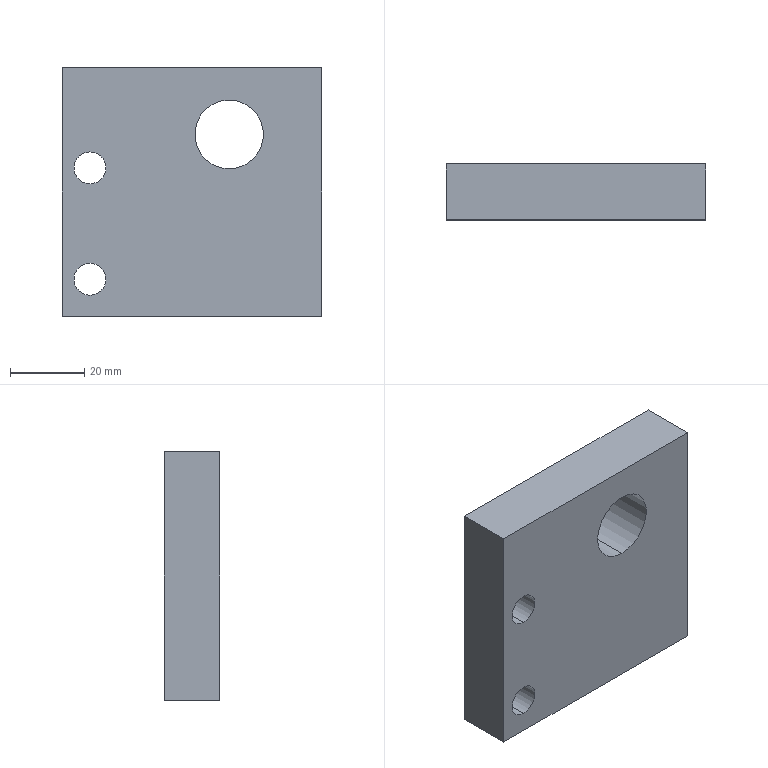Part | 1 solid | 12 faces | box 70 x 15 x 67 mm | volume 64575 mm3 | cylinder 6 | plane 6 | commonest cylinder face diameters 8.6 x4 18.5 x2
STEP:
#1=CARTESIAN_POINT('',(10.,0.,6.25));
#2=VERTEX_POINT('',#1);
#3=CARTESIAN_POINT('',(10.,0.,24.75));
#4=VERTEX_POINT('',#3);
#5=CARTESIAN_POINT('',(10.,0.,15.5));
#6=DIRECTION('',(0.,1.,0.));
#7=DIRECTION('',(0.,0.,1.));
#8=AXIS2_PLACEMENT_3D('',#5,#6,#7);
#9=CIRCLE('',#8,9.25);
#10=EDGE_CURVE('',#2,#4,#9,.T.);
#11=ORIENTED_EDGE('',*,*,#10,.F.);
#12=CARTESIAN_POINT('',(10.,15.,6.25));
#13=VERTEX_POINT('',#12);
#14=CARTESIAN_POINT('',(10.,15.,6.25));
#15=DIRECTION('',(0.,1.,0.));
#16=VECTOR('',#15,1000.);
#17=LINE('',#14,#16);
#18=EDGE_CURVE('',#2,#13,#17,.T.);
#19=ORIENTED_EDGE('',*,*,#18,.T.);
#20=CARTESIAN_POINT('',(10.,15.,24.75));
#21=VERTEX_POINT('',#20);
#22=CARTESIAN_POINT('',(10.,15.,15.5));
#23=DIRECTION('',(0.,1.,0.));
#24=DIRECTION('',(0.,0.,1.));
#25=AXIS2_PLACEMENT_3D('',#22,#23,#24);
#26=CIRCLE('',#25,9.25);
#27=EDGE_CURVE('',#13,#21,#26,.T.);
#28=ORIENTED_EDGE('',*,*,#27,.T.);
#29=CARTESIAN_POINT('',(10.,15.,24.75));
#30=DIRECTION('',(0.,1.,0.));
#31=VECTOR('',#30,1000.);
#32=LINE('',#29,#31);
#33=EDGE_CURVE('',#4,#21,#32,.T.);
#34=ORIENTED_EDGE('',*,*,#33,.F.);
#35=EDGE_LOOP('',(#11,#19,#28,#34));
#36=FACE_OUTER_BOUND('',#35,.T.);
#37=CARTESIAN_POINT('',(10.,15.,15.5));
#38=DIRECTION('',(0.,1.,0.));
#39=DIRECTION('',(0.,0.,1.));
#40=AXIS2_PLACEMENT_3D('',#37,#38,#39);
#41=CYLINDRICAL_SURFACE('',#40,9.25);
#42=ADVANCED_FACE('',(#36),#41,.F.);
#43=CARTESIAN_POINT('',(-27.5,0.,-27.8));
#44=VERTEX_POINT('',#43);
#45=CARTESIAN_POINT('',(-27.5,0.,-19.2));
#46=VERTEX_POINT('',#45);
#47=CARTESIAN_POINT('',(-27.5,0.,-23.5));
#48=DIRECTION('',(0.,1.,0.));
#49=DIRECTION('',(0.,0.,1.));
#50=AXIS2_PLACEMENT_3D('',#47,#48,#49);
#51=CIRCLE('',#50,4.3);
#52=EDGE_CURVE('',#44,#46,#51,.T.);
#53=ORIENTED_EDGE('',*,*,#52,.F.);
#54=CARTESIAN_POINT('',(-27.5,15.,-27.8));
#55=VERTEX_POINT('',#54);
#56=CARTESIAN_POINT('',(-27.5,0.,-27.8));
#57=DIRECTION('',(0.,1.,0.));
#58=VECTOR('',#57,1000.);
#59=LINE('',#56,#58);
#60=EDGE_CURVE('',#44,#55,#59,.T.);
#61=ORIENTED_EDGE('',*,*,#60,.T.);
#62=CARTESIAN_POINT('',(-27.5,15.,-19.2));
#63=VERTEX_POINT('',#62);
#64=CARTESIAN_POINT('',(-27.5,15.,-23.5));
#65=DIRECTION('',(0.,1.,0.));
#66=DIRECTION('',(0.,0.,1.));
#67=AXIS2_PLACEMENT_3D('',#64,#65,#66);
#68=CIRCLE('',#67,4.3);
#69=EDGE_CURVE('',#55,#63,#68,.T.);
#70=ORIENTED_EDGE('',*,*,#69,.T.);
#71=CARTESIAN_POINT('',(-27.5,0.,-19.2));
#72=DIRECTION('',(0.,1.,0.));
#73=VECTOR('',#72,1000.);
#74=LINE('',#71,#73);
#75=EDGE_CURVE('',#46,#63,#74,.T.);
#76=ORIENTED_EDGE('',*,*,#75,.F.);
#77=EDGE_LOOP('',(#53,#61,#70,#76));
#78=FACE_OUTER_BOUND('',#77,.T.);
#79=CARTESIAN_POINT('',(-27.5,0.,-23.5));
#80=DIRECTION('',(0.,1.,0.));
#81=DIRECTION('',(0.,0.,1.));
#82=AXIS2_PLACEMENT_3D('',#79,#80,#81);
#83=CYLINDRICAL_SURFACE('',#82,4.3);
#84=ADVANCED_FACE('',(#78),#83,.F.);
#85=CARTESIAN_POINT('',(-27.5,0.,2.2));
#86=VERTEX_POINT('',#85);
#87=CARTESIAN_POINT('',(-27.5,0.,10.8));
#88=VERTEX_POINT('',#87);
#89=CARTESIAN_POINT('',(-27.5,0.,6.5));
#90=DIRECTION('',(0.,1.,0.));
#91=DIRECTION('',(0.,0.,1.));
#92=AXIS2_PLACEMENT_3D('',#89,#90,#91);
#93=CIRCLE('',#92,4.3);
#94=EDGE_CURVE('',#86,#88,#93,.T.);
#95=ORIENTED_EDGE('',*,*,#94,.F.);
#96=CARTESIAN_POINT('',(-27.5,15.,2.2));
#97=VERTEX_POINT('',#96);
#98=CARTESIAN_POINT('',(-27.5,0.,2.2));
#99=DIRECTION('',(0.,1.,0.));
#100=VECTOR('',#99,1000.);
#101=LINE('',#98,#100);
#102=EDGE_CURVE('',#86,#97,#101,.T.);
#103=ORIENTED_EDGE('',*,*,#102,.T.);
#104=CARTESIAN_POINT('',(-27.5,15.,10.8));
#105=VERTEX_POINT('',#104);
#106=CARTESIAN_POINT('',(-27.5,15.,6.5));
#107=DIRECTION('',(0.,1.,0.));
#108=DIRECTION('',(0.,0.,1.));
#109=AXIS2_PLACEMENT_3D('',#106,#107,#108);
#110=CIRCLE('',#109,4.3);
#111=EDGE_CURVE('',#97,#105,#110,.T.);
#112=ORIENTED_EDGE('',*,*,#111,.T.);
#113=CARTESIAN_POINT('',(-27.5,0.,10.8));
#114=DIRECTION('',(0.,1.,0.));
#115=VECTOR('',#114,1000.);
#116=LINE('',#113,#115);
#117=EDGE_CURVE('',#88,#105,#116,.T.);
#118=ORIENTED_EDGE('',*,*,#117,.F.);
#119=EDGE_LOOP('',(#95,#103,#112,#118));
#120=FACE_OUTER_BOUND('',#119,.T.);
#121=CARTESIAN_POINT('',(-27.5,0.,6.5));
#122=DIRECTION('',(0.,1.,0.));
#123=DIRECTION('',(0.,0.,1.));
#124=AXIS2_PLACEMENT_3D('',#121,#122,#123);
#125=CYLINDRICAL_SURFACE('',#124,4.3);
#126=ADVANCED_FACE('',(#120),#125,.F.);
#127=CARTESIAN_POINT('',(35.,0.,33.5));
#128=VERTEX_POINT('',#127);
#129=CARTESIAN_POINT('',(35.,0.,-33.5));
#130=VERTEX_POINT('',#129);
#131=CARTESIAN_POINT('',(35.,0.,33.5));
#132=DIRECTION('',(0.,0.,-1.));
#133=VECTOR('',#132,1000.);
#134=LINE('',#131,#133);
#135=EDGE_CURVE('',#128,#130,#134,.T.);
#136=ORIENTED_EDGE('',*,*,#135,.T.);
#137=CARTESIAN_POINT('',(35.,15.,-33.5));
#138=VERTEX_POINT('',#137);
#139=CARTESIAN_POINT('',(35.,15.,-33.5));
#140=DIRECTION('',(0.,-1.,0.));
#141=VECTOR('',#140,1000.);
#142=LINE('',#139,#141);
#143=EDGE_CURVE('',#138,#130,#142,.T.);
#144=ORIENTED_EDGE('',*,*,#143,.F.);
#145=CARTESIAN_POINT('',(35.,15.,33.5));
#146=VERTEX_POINT('',#145);
#147=CARTESIAN_POINT('',(35.,15.,33.5));
#148=DIRECTION('',(0.,0.,-1.));
#149=VECTOR('',#148,1000.);
#150=LINE('',#147,#149);
#151=EDGE_CURVE('',#146,#138,#150,.T.);
#152=ORIENTED_EDGE('',*,*,#151,.F.);
#153=CARTESIAN_POINT('',(35.,15.,33.5));
#154=DIRECTION('',(0.,-1.,0.));
#155=VECTOR('',#154,1000.);
#156=LINE('',#153,#155);
#157=EDGE_CURVE('',#146,#128,#156,.T.);
#158=ORIENTED_EDGE('',*,*,#157,.T.);
#159=EDGE_LOOP('',(#136,#144,#152,#158));
#160=FACE_OUTER_BOUND('',#159,.T.);
#161=CARTESIAN_POINT('',(35.,15.,33.5));
#162=DIRECTION('',(-1.,0.,0.));
#163=DIRECTION('',(0.,0.,1.));
#164=AXIS2_PLACEMENT_3D('',#161,#162,#163);
#165=PLANE('',#164);
#166=ADVANCED_FACE('',(#160),#165,.F.);
#167=CARTESIAN_POINT('',(-35.,0.,-33.5));
#168=VERTEX_POINT('',#167);
#169=CARTESIAN_POINT('',(-35.,0.,-33.5));
#170=DIRECTION('',(-1.,0.,0.));
#171=VECTOR('',#170,1000.);
#172=LINE('',#169,#171);
#173=EDGE_CURVE('',#130,#168,#172,.T.);
#174=ORIENTED_EDGE('',*,*,#173,.T.);
#175=CARTESIAN_POINT('',(-35.,15.,-33.5));
#176=VERTEX_POINT('',#175);
#177=CARTESIAN_POINT('',(-35.,15.,-33.5));
#178=DIRECTION('',(0.,-1.,0.));
#179=VECTOR('',#178,1000.);
#180=LINE('',#177,#179);
#181=EDGE_CURVE('',#176,#168,#180,.T.);
#182=ORIENTED_EDGE('',*,*,#181,.F.);
#183=CARTESIAN_POINT('',(-35.,15.,-33.5));
#184=DIRECTION('',(-1.,0.,0.));
#185=VECTOR('',#184,1000.);
#186=LINE('',#183,#185);
#187=EDGE_CURVE('',#138,#176,#186,.T.);
#188=ORIENTED_EDGE('',*,*,#187,.F.);
#189=ORIENTED_EDGE('',*,*,#143,.T.);
#190=EDGE_LOOP('',(#174,#182,#188,#189));
#191=FACE_OUTER_BOUND('',#190,.T.);
#192=CARTESIAN_POINT('',(-35.,15.,-33.5));
#193=DIRECTION('',(0.,0.,1.));
#194=DIRECTION('',(1.,0.,0.));
#195=AXIS2_PLACEMENT_3D('',#192,#193,#194);
#196=PLANE('',#195);
#197=ADVANCED_FACE('',(#191),#196,.F.);
#198=CARTESIAN_POINT('',(-35.,0.,33.5));
#199=VERTEX_POINT('',#198);
#200=CARTESIAN_POINT('',(-35.,0.,33.5));
#201=DIRECTION('',(0.,0.,1.));
#202=VECTOR('',#201,1000.);
#203=LINE('',#200,#202);
#204=EDGE_CURVE('',#168,#199,#203,.T.);
#205=ORIENTED_EDGE('',*,*,#204,.T.);
#206=CARTESIAN_POINT('',(-35.,15.,33.5));
#207=VERTEX_POINT('',#206);
#208=CARTESIAN_POINT('',(-35.,15.,33.5));
#209=DIRECTION('',(0.,-1.,0.));
#210=VECTOR('',#209,1000.);
#211=LINE('',#208,#210);
#212=EDGE_CURVE('',#207,#199,#211,.T.);
#213=ORIENTED_EDGE('',*,*,#212,.F.);
#214=CARTESIAN_POINT('',(-35.,15.,33.5));
#215=DIRECTION('',(0.,0.,1.));
#216=VECTOR('',#215,1000.);
#217=LINE('',#214,#216);
#218=EDGE_CURVE('',#176,#207,#217,.T.);
#219=ORIENTED_EDGE('',*,*,#218,.F.);
#220=ORIENTED_EDGE('',*,*,#181,.T.);
#221=EDGE_LOOP('',(#205,#213,#219,#220));
#222=FACE_OUTER_BOUND('',#221,.T.);
#223=CARTESIAN_POINT('',(-35.,15.,33.5));
#224=DIRECTION('',(1.,0.,0.));
#225=DIRECTION('',(0.,0.,-1.));
#226=AXIS2_PLACEMENT_3D('',#223,#224,#225);
#227=PLANE('',#226);
#228=ADVANCED_FACE('',(#222),#227,.F.);
#229=CARTESIAN_POINT('',(-35.,0.,33.5));
#230=DIRECTION('',(1.,0.,0.));
#231=VECTOR('',#230,1000.);
#232=LINE('',#229,#231);
#233=EDGE_CURVE('',#199,#128,#232,.T.);
#234=ORIENTED_EDGE('',*,*,#233,.T.);
#235=ORIENTED_EDGE('',*,*,#157,.F.);
#236=CARTESIAN_POINT('',(-35.,15.,33.5));
#237=DIRECTION('',(1.,0.,0.));
#238=VECTOR('',#237,1000.);
#239=LINE('',#236,#238);
#240=EDGE_CURVE('',#207,#146,#239,.T.);
#241=ORIENTED_EDGE('',*,*,#240,.F.);
#242=ORIENTED_EDGE('',*,*,#212,.T.);
#243=EDGE_LOOP('',(#234,#235,#241,#242));
#244=FACE_OUTER_BOUND('',#243,.T.);
#245=CARTESIAN_POINT('',(-35.,15.,33.5));
#246=DIRECTION('',(0.,0.,-1.));
#247=DIRECTION('',(-1.,0.,0.));
#248=AXIS2_PLACEMENT_3D('',#245,#246,#247);
#249=PLANE('',#248);
#250=ADVANCED_FACE('',(#244),#249,.F.);
#251=CARTESIAN_POINT('',(10.,15.,15.5));
#252=DIRECTION('',(0.,1.,0.));
#253=DIRECTION('',(0.,0.,1.));
#254=AXIS2_PLACEMENT_3D('',#251,#252,#253);
#255=CIRCLE('',#254,9.25);
#256=EDGE_CURVE('',#21,#13,#255,.T.);
#257=ORIENTED_EDGE('',*,*,#256,.F.);
#258=ORIENTED_EDGE('',*,*,#27,.F.);
#259=EDGE_LOOP('',(#257,#258));
#260=FACE_BOUND('',#259,.T.);
#261=CARTESIAN_POINT('',(-27.5,15.,-23.5));
#262=DIRECTION('',(0.,1.,0.));
#263=DIRECTION('',(0.,0.,1.));
#264=AXIS2_PLACEMENT_3D('',#261,#262,#263);
#265=CIRCLE('',#264,4.3);
#266=EDGE_CURVE('',#63,#55,#265,.T.);
#267=ORIENTED_EDGE('',*,*,#266,.F.);
#268=ORIENTED_EDGE('',*,*,#69,.F.);
#269=EDGE_LOOP('',(#267,#268));
#270=FACE_BOUND('',#269,.T.);
#271=CARTESIAN_POINT('',(-27.5,15.,6.5));
#272=DIRECTION('',(0.,1.,0.));
#273=DIRECTION('',(0.,0.,1.));
#274=AXIS2_PLACEMENT_3D('',#271,#272,#273);
#275=CIRCLE('',#274,4.3);
#276=EDGE_CURVE('',#105,#97,#275,.T.);
#277=ORIENTED_EDGE('',*,*,#276,.F.);
#278=ORIENTED_EDGE('',*,*,#111,.F.);
#279=EDGE_LOOP('',(#277,#278));
#280=FACE_BOUND('',#279,.T.);
#281=ORIENTED_EDGE('',*,*,#151,.T.);
#282=ORIENTED_EDGE('',*,*,#187,.T.);
#283=ORIENTED_EDGE('',*,*,#218,.T.);
#284=ORIENTED_EDGE('',*,*,#240,.T.);
#285=EDGE_LOOP('',(#281,#282,#283,#284));
#286=FACE_OUTER_BOUND('',#285,.T.);
#287=CARTESIAN_POINT('',(0.,15.,0.));
#288=DIRECTION('',(0.,-1.,0.));
#289=DIRECTION('',(0.,0.,-1.));
#290=AXIS2_PLACEMENT_3D('',#287,#288,#289);
#291=PLANE('',#290);
#292=ADVANCED_FACE('',(#260,#270,#280,#286),#291,.F.);
#293=CARTESIAN_POINT('',(10.,0.,15.5));
#294=DIRECTION('',(0.,1.,0.));
#295=DIRECTION('',(0.,0.,1.));
#296=AXIS2_PLACEMENT_3D('',#293,#294,#295);
#297=CIRCLE('',#296,9.25);
#298=EDGE_CURVE('',#4,#2,#297,.T.);
#299=ORIENTED_EDGE('',*,*,#298,.T.);
#300=ORIENTED_EDGE('',*,*,#10,.T.);
#301=EDGE_LOOP('',(#299,#300));
#302=FACE_BOUND('',#301,.T.);
#303=CARTESIAN_POINT('',(-27.5,0.,-23.5));
#304=DIRECTION('',(0.,1.,0.));
#305=DIRECTION('',(0.,0.,1.));
#306=AXIS2_PLACEMENT_3D('',#303,#304,#305);
#307=CIRCLE('',#306,4.3);
#308=EDGE_CURVE('',#46,#44,#307,.T.);
#309=ORIENTED_EDGE('',*,*,#308,.T.);
#310=ORIENTED_EDGE('',*,*,#52,.T.);
#311=EDGE_LOOP('',(#309,#310));
#312=FACE_BOUND('',#311,.T.);
#313=CARTESIAN_POINT('',(-27.5,0.,6.5));
#314=DIRECTION('',(0.,1.,0.));
#315=DIRECTION('',(0.,0.,1.));
#316=AXIS2_PLACEMENT_3D('',#313,#314,#315);
#317=CIRCLE('',#316,4.3);
#318=EDGE_CURVE('',#88,#86,#317,.T.);
#319=ORIENTED_EDGE('',*,*,#318,.T.);
#320=ORIENTED_EDGE('',*,*,#94,.T.);
#321=EDGE_LOOP('',(#319,#320));
#322=FACE_BOUND('',#321,.T.);
#323=ORIENTED_EDGE('',*,*,#135,.F.);
#324=ORIENTED_EDGE('',*,*,#233,.F.);
#325=ORIENTED_EDGE('',*,*,#204,.F.);
#326=ORIENTED_EDGE('',*,*,#173,.F.);
#327=EDGE_LOOP('',(#323,#324,#325,#326));
#328=FACE_OUTER_BOUND('',#327,.T.);
#329=CARTESIAN_POINT('',(0.,0.,0.));
#330=DIRECTION('',(0.,-1.,0.));
#331=DIRECTION('',(0.,0.,-1.));
#332=AXIS2_PLACEMENT_3D('',#329,#330,#331);
#333=PLANE('',#332);
#334=ADVANCED_FACE('',(#302,#312,#322,#328),#333,.T.);
#335=ORIENTED_EDGE('',*,*,#102,.F.);
#336=ORIENTED_EDGE('',*,*,#318,.F.);
#337=ORIENTED_EDGE('',*,*,#117,.T.);
#338=ORIENTED_EDGE('',*,*,#276,.T.);
#339=EDGE_LOOP('',(#335,#336,#337,#338));
#340=FACE_OUTER_BOUND('',#339,.T.);
#341=CARTESIAN_POINT('',(-27.5,0.,6.5));
#342=DIRECTION('',(0.,1.,0.));
#343=DIRECTION('',(0.,0.,1.));
#344=AXIS2_PLACEMENT_3D('',#341,#342,#343);
#345=CYLINDRICAL_SURFACE('',#344,4.3);
#346=ADVANCED_FACE('',(#340),#345,.F.);
#347=ORIENTED_EDGE('',*,*,#60,.F.);
#348=ORIENTED_EDGE('',*,*,#308,.F.);
#349=ORIENTED_EDGE('',*,*,#75,.T.);
#350=ORIENTED_EDGE('',*,*,#266,.T.);
#351=EDGE_LOOP('',(#347,#348,#349,#350));
#352=FACE_OUTER_BOUND('',#351,.T.);
#353=CARTESIAN_POINT('',(-27.5,0.,-23.5));
#354=DIRECTION('',(0.,1.,0.));
#355=DIRECTION('',(0.,0.,1.));
#356=AXIS2_PLACEMENT_3D('',#353,#354,#355);
#357=CYLINDRICAL_SURFACE('',#356,4.3);
#358=ADVANCED_FACE('',(#352),#357,.F.);
#359=ORIENTED_EDGE('',*,*,#18,.F.);
#360=ORIENTED_EDGE('',*,*,#298,.F.);
#361=ORIENTED_EDGE('',*,*,#33,.T.);
#362=ORIENTED_EDGE('',*,*,#256,.T.);
#363=EDGE_LOOP('',(#359,#360,#361,#362));
#364=FACE_OUTER_BOUND('',#363,.T.);
#365=CARTESIAN_POINT('',(10.,15.,15.5));
#366=DIRECTION('',(0.,1.,0.));
#367=DIRECTION('',(0.,0.,1.));
#368=AXIS2_PLACEMENT_3D('',#365,#366,#367);
#369=CYLINDRICAL_SURFACE('',#368,9.25);
#370=ADVANCED_FACE('',(#364),#369,.F.);
#371=CLOSED_SHELL('',(#42,#84,#126,#166,#197,#228,#250,#292,#334,#346,#358,#370));
#372=MANIFOLD_SOLID_BREP('',#371);
#373=CARTESIAN_POINT('',(0.,0.,0.));
#374=DIRECTION('',(0.,0.,1.));
#375=DIRECTION('',(1.,0.,0.));
#376=AXIS2_PLACEMENT_3D('',#373,#374,#375);
#377=(LENGTH_UNIT()NAMED_UNIT(*)SI_UNIT(.MILLI.,.METRE.));
#378=UNCERTAINTY_MEASURE_WITH_UNIT(LENGTH_MEASURE(0.00001),#377,'','');
#379=(NAMED_UNIT(*)PLANE_ANGLE_UNIT()SI_UNIT($,.RADIAN.));
#380=(NAMED_UNIT(*)SI_UNIT($,.STERADIAN.)SOLID_ANGLE_UNIT());
#381=(GEOMETRIC_REPRESENTATION_CONTEXT(3)GLOBAL_UNCERTAINTY_ASSIGNED_CONTEXT((#378))GLOBAL_UNIT_ASSIGNED_CONTEXT((#377,#379,#380))REPRESENTATION_CONTEXT('',''));
#382=ADVANCED_BREP_SHAPE_REPRESENTATION('',(#372,#376),#381);